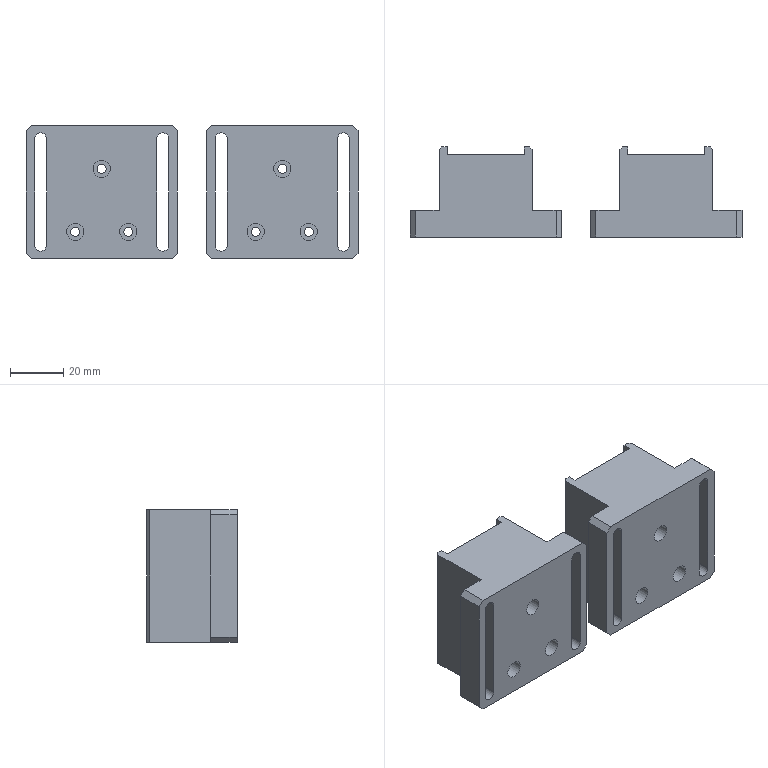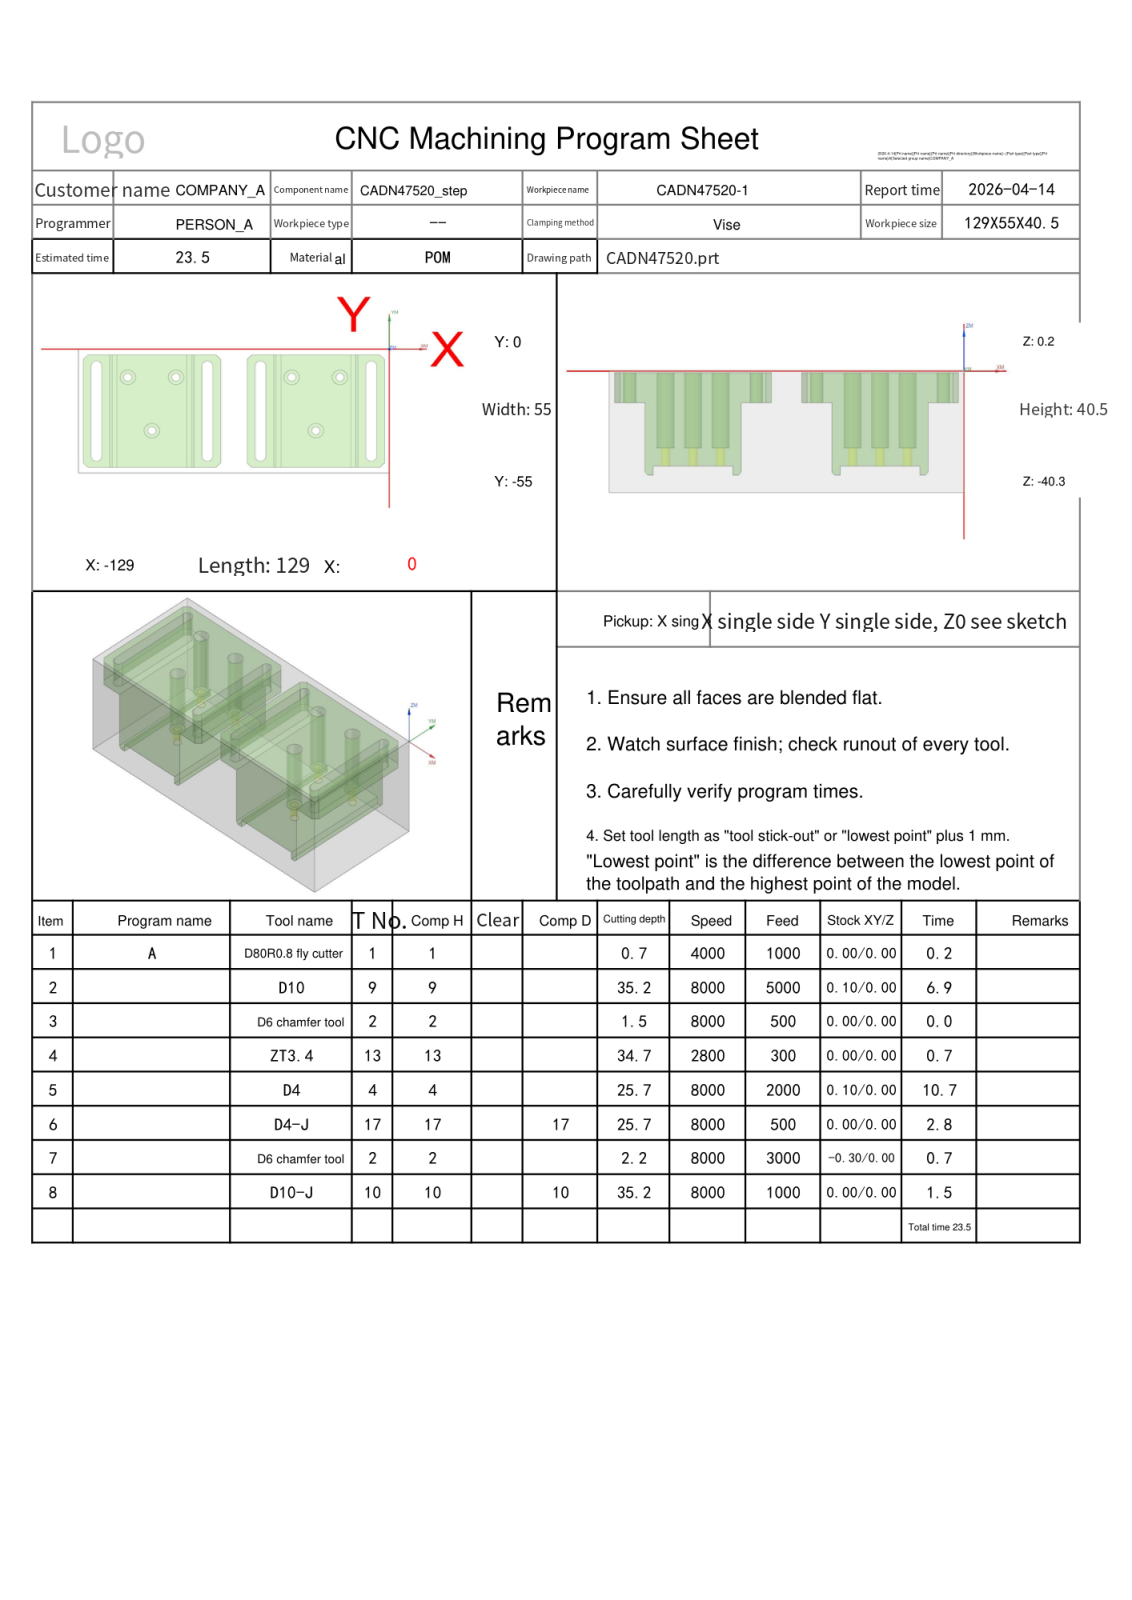NC program | NX | posted by the shop | part box 125 x 34 x 50 mm
Lines 2381 to 3331 of 5259:
N5 T04 M06
(D4  D=4. R=0. H=04 ce=0.10 di=0.10)
G00 G90 G54 X-7.65 Y-27.5 M03 S8000
G43 H04 Z19.5
M08
Z0.0
G01 Y-47.5 Z-.06 F2500.
G03 X-7.5 Y-47.65 Z-.061 I.15 J0.0
X-7.35 Y-47.5 Z-.062 I0.0 J.15
G01 Y-7.5 Z-.183
G03 X-7.5 Y-7.35 Z-.183 I-.15 J0.0
X-7.65 Y-7.5 Z-.184 I0.0 J-.15
G01 Y-47.5 Z-.305
G03 X-7.5 Y-47.65 Z-.306 I.15 J0.0
X-7.35 Y-47.5 Z-.306 I0.0 J.15
G01 Y-7.5 Z-.427
G03 X-7.5 Y-7.35 Z-.428 I-.15 J0.0
X-7.65 Y-7.5 Z-.428 I0.0 J-.15
G01 Y-47.5 Z-.549
G03 X-7.5 Y-47.65 Z-.55 I.15 J0.0
X-7.35 Y-47.5 Z-.551 I0.0 J.15
G01 Y-7.5 Z-.672
G03 X-7.5 Y-7.35 Z-.672 I-.15 J0.0
X-7.65 Y-7.5 Z-.673 I0.0 J-.15
G01 Y-47.5 Z-.794
G03 X-7.5 Y-47.65 Z-.794 I.15 J0.0
X-7.35 Y-47.5 Z-.795 I0.0 J.15
G01 Y-7.5 Z-.916
G03 X-7.5 Y-7.35 Z-.917 I-.15 J0.0
X-7.65 Y-7.5 Z-.917 I0.0 J-.15
G01 Y-47.5 Z-1.038
G03 X-7.5 Y-47.65 Z-1.039 I.15 J0.0
X-7.35 Y-47.5 Z-1.04 I0.0 J.15
G01 Y-7.5 Z-1.16
G03 X-7.5 Y-7.35 Z-1.161 I-.15 J0.0
X-7.65 Y-7.5 Z-1.162 I0.0 J-.15
G01 Y-47.5 Z-1.283
G03 X-7.5 Y-47.65 Z-1.283 I.15 J0.0
X-7.35 Y-47.5 Z-1.284 I0.0 J.15
G01 Y-7.5 Z-1.405
G03 X-7.5 Y-7.35 Z-1.406 I-.15 J0.0
X-7.65 Y-7.5 Z-1.406 I0.0 J-.15
G01 Y-47.5 Z-1.527
G03 X-7.5 Y-47.65 Z-1.528 I.15 J0.0
X-7.35 Y-47.5 Z-1.528 I0.0 J.15
G01 Y-7.5 Z-1.649
G03 X-7.5 Y-7.35 Z-1.65 I-.15 J0.0
X-7.65 Y-7.5 Z-1.651 I0.0 J-.15
G01 Y-47.5 Z-1.772
G03 X-7.5 Y-47.65 Z-1.772 I.15 J0.0
X-7.35 Y-47.5 Z-1.773 I0.0 J.15
G01 Y-7.5 Z-1.894
G03 X-7.5 Y-7.35 Z-1.894 I-.15 J0.0
X-7.65 Y-7.5 Z-1.895 I0.0 J-.15
G01 Y-47.5 Z-2.016
G03 X-7.5 Y-47.65 Z-2.017 I.15 J0.0
X-7.35 Y-47.5 Z-2.017 I0.0 J.15
G01 Y-7.5 Z-2.138
G03 X-7.5 Y-7.35 Z-2.139 I-.15 J0.0
X-7.65 Y-7.5 Z-2.14 I0.0 J-.15
G01 Y-47.5 Z-2.26
G03 X-7.5 Y-47.65 Z-2.261 I.15 J0.0
X-7.35 Y-47.5 Z-2.262 I0.0 J.15
G01 Y-7.5 Z-2.383
G03 X-7.5 Y-7.35 Z-2.383 I-.15 J0.0
X-7.65 Y-7.5 Z-2.384 I0.0 J-.15
G01 Y-47.5 Z-2.505
G03 X-7.5 Y-47.65 Z-2.506 I.15 J0.0
X-7.35 Y-47.5 Z-2.506 I0.0 J.15
G01 Y-7.5 Z-2.627
G03 X-7.5 Y-7.35 Z-2.628 I-.15 J0.0
X-7.65 Y-7.5 Z-2.628 I0.0 J-.15
G01 Y-47.5 Z-2.749
G03 X-7.5 Y-47.65 Z-2.75 I.15 J0.0
X-7.35 Y-47.5 Z-2.751 I0.0 J.15
G01 Y-7.5 Z-2.872
G03 X-7.5 Y-7.35 Z-2.872 I-.15 J0.0
X-7.65 Y-7.5 Z-2.873 I0.0 J-.15
G01 Y-47.5 Z-2.994
G03 X-7.5 Y-47.65 Z-2.994 I.15 J0.0
X-7.35 Y-47.5 Z-2.995 I0.0 J.15
G01 Y-7.5 Z-3.116
G03 X-7.5 Y-7.35 Z-3.117 I-.15 J0.0
X-7.65 Y-7.5 Z-3.117 I0.0 J-.15
G01 Y-47.5 Z-3.238
G03 X-7.5 Y-47.65 Z-3.239 I.15 J0.0
X-7.35 Y-47.5 Z-3.24 I0.0 J.15
G01 Y-7.5 Z-3.36
G03 X-7.5 Y-7.35 Z-3.361 I-.15 J0.0
X-7.65 Y-7.5 Z-3.362 I0.0 J-.15
G01 Y-47.5 Z-3.483
G03 X-7.5 Y-47.65 Z-3.483 I.15 J0.0
X-7.35 Y-47.5 Z-3.484 I0.0 J.15
G01 Y-7.5 Z-3.605
G03 X-7.5 Y-7.35 Z-3.606 I-.15 J0.0
X-7.65 Y-7.5 Z-3.606 I0.0 J-.15
G01 Y-47.5 Z-3.727
G03 X-7.5 Y-47.65 Z-3.728 I.15 J0.0
X-7.35 Y-47.5 Z-3.728 I0.0 J.15
G01 Y-7.5 Z-3.849
G03 X-7.5 Y-7.35 Z-3.85 I-.15 J0.0
X-7.65 Y-7.5 Z-3.851 I0.0 J-.15
G01 Y-47.5 Z-3.972
G03 X-7.5 Y-47.65 Z-3.972 I.15 J0.0
X-7.35 Y-47.5 Z-3.973 I0.0 J.15
G01 Y-7.5 Z-4.094
G03 X-7.5 Y-7.35 Z-4.094 I-.15 J0.0
X-7.65 Y-7.5 Z-4.095 I0.0 J-.15
G01 Y-47.5 Z-4.216
G03 X-7.5 Y-47.65 Z-4.217 I.15 J0.0
X-7.35 Y-47.5 Z-4.217 I0.0 J.15
G01 Y-7.5 Z-4.338
G03 X-7.5 Y-7.35 Z-4.339 I-.15 J0.0
X-7.65 Y-7.5 Z-4.34 I0.0 J-.15
G01 Y-47.5 Z-4.46
G03 X-7.5 Y-47.65 Z-4.461 I.15 J0.0
X-7.35 Y-47.5 Z-4.462 I0.0 J.15
G01 Y-7.5 Z-4.583
G03 X-7.5 Y-7.35 Z-4.583 I-.15 J0.0
X-7.65 Y-7.5 Z-4.584 I0.0 J-.15
G01 Y-47.5 Z-4.705
G03 X-7.5 Y-47.65 Z-4.706 I.15 J0.0
X-7.35 Y-47.5 Z-4.706 I0.0 J.15
G01 Y-7.5 Z-4.827
G03 X-7.5 Y-7.35 Z-4.828 I-.15 J0.0
X-7.65 Y-7.5 Z-4.828 I0.0 J-.15
G01 Y-47.5 Z-4.949
G03 X-7.5 Y-47.65 Z-4.95 I.15 J0.0
X-7.35 Y-47.5 Z-4.951 I0.0 J.15
G01 Y-7.5 Z-5.072
G03 X-7.5 Y-7.35 Z-5.072 I-.15 J0.0
X-7.65 Y-7.5 Z-5.073 I0.0 J-.15
G01 Y-47.5 Z-5.194
G03 X-7.5 Y-47.65 Z-5.194 I.15 J0.0
X-7.35 Y-47.5 Z-5.195 I0.0 J.15
G01 Y-7.5 Z-5.316
G03 X-7.5 Y-7.35 Z-5.317 I-.15 J0.0
X-7.65 Y-7.5 Z-5.317 I0.0 J-.15
G01 Y-47.5 Z-5.438
G03 X-7.5 Y-47.65 Z-5.439 I.15 J0.0
X-7.35 Y-47.5 Z-5.44 I0.0 J.15
G01 Y-7.5 Z-5.56
G03 X-7.5 Y-7.35 Z-5.561 I-.15 J0.0
X-7.65 Y-7.5 Z-5.562 I0.0 J-.15
G01 Y-47.5 Z-5.683
G03 X-7.5 Y-47.65 Z-5.683 I.15 J0.0
X-7.35 Y-47.5 Z-5.684 I0.0 J.15
G01 Y-7.5 Z-5.805
G03 X-7.5 Y-7.35 Z-5.806 I-.15 J0.0
X-7.65 Y-7.5 Z-5.806 I0.0 J-.15
G01 Y-47.5 Z-5.927
G03 X-7.5 Y-47.65 Z-5.928 I.15 J0.0
X-7.35 Y-47.5 Z-5.928 I0.0 J.15
G01 Y-7.5 Z-6.049
G03 X-7.5 Y-7.35 Z-6.05 I-.15 J0.0
X-7.65 Y-7.5 Z-6.051 I0.0 J-.15
G01 Y-47.5 Z-6.172
G03 X-7.5 Y-47.65 Z-6.172 I.15 J0.0
X-7.35 Y-47.5 Z-6.173 I0.0 J.15
G01 Y-7.5 Z-6.294
G03 X-7.5 Y-7.35 Z-6.294 I-.15 J0.0
X-7.65 Y-7.5 Z-6.295 I0.0 J-.15
G01 Y-47.5 Z-6.416
G03 X-7.5 Y-47.65 Z-6.417 I.15 J0.0
X-7.35 Y-47.5 Z-6.417 I0.0 J.15
G01 Y-7.5 Z-6.538
G03 X-7.5 Y-7.35 Z-6.539 I-.15 J0.0
X-7.65 Y-7.5 Z-6.54 I0.0 J-.15
G01 Y-47.5 Z-6.66
G03 X-7.5 Y-47.65 Z-6.661 I.15 J0.0
X-7.35 Y-47.5 Z-6.662 I0.0 J.15
G01 Y-7.5 Z-6.783
G03 X-7.5 Y-7.35 Z-6.783 I-.15 J0.0
X-7.65 Y-7.5 Z-6.784 I0.0 J-.15
G01 Y-47.5 Z-6.905
G03 X-7.5 Y-47.65 Z-6.906 I.15 J0.0
X-7.35 Y-47.5 Z-6.906 I0.0 J.15
G01 Y-7.5 Z-7.027
G03 X-7.5 Y-7.35 Z-7.028 I-.15 J0.0
X-7.65 Y-7.5 Z-7.028 I0.0 J-.15
G01 Y-47.5 Z-7.149
G03 X-7.5 Y-47.65 Z-7.15 I.15 J0.0
X-7.35 Y-47.5 Z-7.151 I0.0 J.15
G01 Y-7.5 Z-7.272
G03 X-7.5 Y-7.35 Z-7.272 I-.15 J0.0
X-7.65 Y-7.5 Z-7.273 I0.0 J-.15
G01 Y-47.5 Z-7.394
G03 X-7.5 Y-47.65 Z-7.394 I.15 J0.0
X-7.35 Y-47.5 Z-7.395 I0.0 J.15
G01 Y-7.5 Z-7.516
G03 X-7.5 Y-7.35 Z-7.517 I-.15 J0.0
X-7.65 Y-7.5 Z-7.517 I0.0 J-.15
G01 Y-47.5 Z-7.638
G03 X-7.5 Y-47.65 Z-7.639 I.15 J0.0
X-7.35 Y-47.5 Z-7.64 I0.0 J.15
G01 Y-7.5 Z-7.76
G03 X-7.5 Y-7.35 Z-7.761 I-.15 J0.0
X-7.65 Y-7.5 Z-7.762 I0.0 J-.15
G01 Y-47.5 Z-7.883
G03 X-7.5 Y-47.65 Z-7.883 I.15 J0.0
X-7.35 Y-47.5 Z-7.884 I0.0 J.15
G01 Y-7.5 Z-8.005
G03 X-7.5 Y-7.35 Z-8.006 I-.15 J0.0
X-7.65 Y-7.5 Z-8.006 I0.0 J-.15
G01 Y-47.5 Z-8.127
G03 X-7.5 Y-47.65 Z-8.128 I.15 J0.0
X-7.35 Y-47.5 Z-8.128 I0.0 J.15
G01 Y-7.5 Z-8.249
G03 X-7.5 Y-7.35 Z-8.25 I-.15 J0.0
X-7.65 Y-7.5 Z-8.251 I0.0 J-.15
G01 Y-47.5 Z-8.372
G03 X-7.5 Y-47.65 Z-8.372 I.15 J0.0
X-7.35 Y-47.5 Z-8.373 I0.0 J.15
G01 Y-7.5 Z-8.494
G03 X-7.5 Y-7.35 Z-8.494 I-.15 J0.0
X-7.65 Y-7.5 Z-8.495 I0.0 J-.15
G01 Y-47.5 Z-8.616
G03 X-7.5 Y-47.65 Z-8.617 I.15 J0.0
X-7.35 Y-47.5 Z-8.617 I0.0 J.15
G01 Y-7.5 Z-8.738
G03 X-7.5 Y-7.35 Z-8.739 I-.15 J0.0
X-7.65 Y-7.5 Z-8.74 I0.0 J-.15
G01 Y-47.5 Z-8.86
G03 X-7.5 Y-47.65 Z-8.861 I.15 J0.0
X-7.35 Y-47.5 Z-8.862 I0.0 J.15
G01 Y-7.5 Z-8.983
G03 X-7.5 Y-7.35 Z-8.983 I-.15 J0.0
X-7.65 Y-7.5 Z-8.984 I0.0 J-.15
G01 Y-47.5 Z-9.105
G03 X-7.5 Y-47.65 Z-9.106 I.15 J0.0
X-7.35 Y-47.5 Z-9.106 I0.0 J.15
G01 Y-7.5 Z-9.227
G03 X-7.5 Y-7.35 Z-9.228 I-.15 J0.0
X-7.65 Y-7.5 Z-9.228 I0.0 J-.15
G01 Y-47.5 Z-9.349
G03 X-7.5 Y-47.65 Z-9.35 I.15 J0.0
X-7.35 Y-47.5 Z-9.351 I0.0 J.15
G01 Y-7.5 Z-9.472
G03 X-7.5 Y-7.35 Z-9.472 I-.15 J0.0
X-7.65 Y-7.5 Z-9.473 I0.0 J-.15
G01 Y-47.5 Z-9.594
G03 X-7.5 Y-47.65 Z-9.594 I.15 J0.0
X-7.35 Y-47.5 Z-9.595 I0.0 J.15
G01 Y-7.5 Z-9.716
G03 X-7.5 Y-7.35 Z-9.717 I-.15 J0.0
X-7.65 Y-7.5 Z-9.717 I0.0 J-.15
G01 Y-47.5 Z-9.838
G03 X-7.5 Y-47.65 Z-9.839 I.15 J0.0
X-7.35 Y-47.5 Z-9.84 I0.0 J.15
G01 Y-7.5 Z-9.96
G03 X-7.5 Y-7.35 Z-9.961 I-.15 J0.0
X-7.65 Y-7.5 Z-9.962 I0.0 J-.15
G01 Y-47.5 Z-10.083
G03 X-7.5 Y-47.65 Z-10.083 I.15 J0.0
X-7.35 Y-47.5 Z-10.084 I0.0 J.15
G01 Y-7.5 Z-10.205
G03 X-7.5 Y-7.35 Z-10.206 I-.15 J0.0
X-7.65 Y-7.5 Z-10.206 I0.0 J-.15
G01 Y-47.5 Z-10.327
G03 X-7.5 Y-47.65 Z-10.328 I.15 J0.0
X-7.35 Y-47.5 Z-10.328 I0.0 J.15
G01 Y-7.5 Z-10.449
G03 X-7.5 Y-7.35 Z-10.45 I-.15 J0.0
X-7.65 Y-7.5 Z-10.451 I0.0 J-.15
G01 Y-47.5 Z-10.572
G03 X-7.5 Y-47.65 Z-10.572 I.15 J0.0
X-7.35 Y-47.5 Z-10.573 I0.0 J.15
G01 Y-7.5 Z-10.694
G03 X-7.5 Y-7.35 Z-10.694 I-.15 J0.0
X-7.65 Y-7.5 Z-10.695 I0.0 J-.15
G01 Y-47.5 Z-10.816
G03 X-7.5 Y-47.65 Z-10.817 I.15 J0.0
X-7.35 Y-47.5 Z-10.817 I0.0 J.15
G01 Y-7.5 Z-10.938
G03 X-7.5 Y-7.35 Z-10.939 I-.15 J0.0
X-7.65 Y-7.5 Z-10.94 I0.0 J-.15
G01 Y-27.5 Z-11.
Y-47.5
G03 X-7.5 Y-47.65 I.15 J0.0
X-7.35 Y-47.5 I0.0 J.15
G01 Y-7.5
G03 X-7.5 Y-7.35 I-.15 J0.0
X-7.65 Y-7.5 I0.0 J-.15
G01 Y-27.5
Y-28.
Z-10.
G00 Z19.5
X-53.65 Y-27.5
Z0.0
G01 Y-47.5 Z-.06
G03 X-53.5 Y-47.65 Z-.061 I.15 J0.0
X-53.35 Y-47.5 Z-.062 I0.0 J.15
G01 Y-7.5 Z-.183
Y-7.445
X-53.378 Y-7.397
X-53.425 Y-7.37
X-53.459 Y-7.345
X-53.5 Y-7.35
G03 X-53.65 Y-7.5 Z-.184 I0.0 J-.15
G01 Y-47.5 Z-.305
G03 X-53.5 Y-47.65 Z-.306 I.15 J0.0
X-53.35 Y-47.5 Z-.306 I0.0 J.15
G01 Y-7.5 Z-.427
Y-7.445
X-53.378 Y-7.397
X-53.425 Y-7.37 Z-.428
X-53.459 Y-7.345
X-53.5 Y-7.35
G03 X-53.65 Y-7.5 Z-.428 I0.0 J-.15
G01 Y-47.5 Z-.549
G03 X-53.5 Y-47.65 Z-.55 I.15 J0.0
X-53.35 Y-47.5 Z-.551 I0.0 J.15
G01 Y-7.5 Z-.672
Y-7.445
X-53.378 Y-7.397
X-53.425 Y-7.37
X-53.459 Y-7.345
X-53.5 Y-7.35
G03 X-53.65 Y-7.5 Z-.673 I0.0 J-.15
G01 Y-47.5 Z-.794
G03 X-53.5 Y-47.65 Z-.794 I.15 J0.0
X-53.35 Y-47.5 Z-.795 I0.0 J.15
G01 Y-7.5 Z-.916
Y-7.445
X-53.378 Y-7.397
X-53.425 Y-7.37
X-53.459 Y-7.345 Z-.917
X-53.5 Y-7.35
G03 X-53.65 Y-7.5 Z-.917 I0.0 J-.15
G01 Y-47.5 Z-1.038
G03 X-53.5 Y-47.65 Z-1.039 I.15 J0.0
X-53.35 Y-47.5 Z-1.04 I0.0 J.15
G01 Y-7.5 Z-1.16
Y-7.445 Z-1.161
X-53.378 Y-7.397
X-53.425 Y-7.37
X-53.459 Y-7.345
X-53.5 Y-7.35
G03 X-53.65 Y-7.5 Z-1.162 I0.0 J-.15
G01 Y-47.5 Z-1.283
G03 X-53.5 Y-47.65 Z-1.283 I.15 J0.0
X-53.35 Y-47.5 Z-1.284 I0.0 J.15
G01 Y-7.5 Z-1.405
Y-7.445
X-53.378 Y-7.397
X-53.425 Y-7.37
X-53.459 Y-7.345
X-53.5 Y-7.35 Z-1.406
G03 X-53.65 Y-7.5 Z-1.406 I0.0 J-.15
G01 Y-47.5 Z-1.527
G03 X-53.5 Y-47.65 Z-1.528 I.15 J0.0
X-53.35 Y-47.5 Z-1.528 I0.0 J.15
G01 Y-7.5 Z-1.649
Y-7.445
X-53.378 Y-7.397 Z-1.65
X-53.425 Y-7.37
X-53.459 Y-7.345
X-53.5 Y-7.35
G03 X-53.65 Y-7.5 Z-1.651 I0.0 J-.15
G01 Y-47.5 Z-1.772
G03 X-53.5 Y-47.65 Z-1.772 I.15 J0.0
X-53.35 Y-47.5 Z-1.773 I0.0 J.15
G01 Y-7.5 Z-1.894
Y-7.445
X-53.378 Y-7.397
X-53.425 Y-7.37
X-53.459 Y-7.345
X-53.5 Y-7.35
G03 X-53.65 Y-7.5 Z-1.895 I0.0 J-.15
G01 Y-47.5 Z-2.016
G03 X-53.5 Y-47.65 Z-2.017 I.15 J0.0
X-53.35 Y-47.5 Z-2.017 I0.0 J.15
G01 Y-7.5 Z-2.138
Y-7.445
X-53.378 Y-7.397
X-53.425 Y-7.37 Z-2.139
X-53.459 Y-7.345
X-53.5 Y-7.35
G03 X-53.65 Y-7.5 Z-2.14 I0.0 J-.15
G01 Y-47.5 Z-2.26
G03 X-53.5 Y-47.65 Z-2.261 I.15 J0.0
X-53.35 Y-47.5 Z-2.262 I0.0 J.15
G01 Y-7.5 Z-2.383
Y-7.445
X-53.378 Y-7.397
X-53.425 Y-7.37
X-53.459 Y-7.345
X-53.5 Y-7.35
G03 X-53.65 Y-7.5 Z-2.384 I0.0 J-.15
G01 Y-47.5 Z-2.505
G03 X-53.5 Y-47.65 Z-2.506 I.15 J0.0
X-53.35 Y-47.5 Z-2.506 I0.0 J.15
G01 Y-7.5 Z-2.627
Y-7.445
X-53.378 Y-7.397
X-53.425 Y-7.37 Z-2.628
X-53.459 Y-7.345
X-53.5 Y-7.35
G03 X-53.65 Y-7.5 Z-2.628 I0.0 J-.15
G01 Y-47.5 Z-2.749
G03 X-53.5 Y-47.65 Z-2.75 I.15 J0.0
X-53.35 Y-47.5 Z-2.751 I0.0 J.15
G01 Y-7.5 Z-2.872
Y-7.445
X-53.378 Y-7.397
X-53.425 Y-7.37
X-53.459 Y-7.345
X-53.5 Y-7.35
G03 X-53.65 Y-7.5 Z-2.873 I0.0 J-.15
G01 Y-47.5 Z-2.994
G03 X-53.5 Y-47.65 Z-2.994 I.15 J0.0
X-53.35 Y-47.5 Z-2.995 I0.0 J.15
G01 Y-7.5 Z-3.116
Y-7.445
X-53.378 Y-7.397
X-53.425 Y-7.37
X-53.459 Y-7.345 Z-3.117
X-53.5 Y-7.35
G03 X-53.65 Y-7.5 Z-3.117 I0.0 J-.15
G01 Y-47.5 Z-3.238
G03 X-53.5 Y-47.65 Z-3.239 I.15 J0.0
X-53.35 Y-47.5 Z-3.24 I0.0 J.15
G01 Y-7.5 Z-3.36
Y-7.445 Z-3.361
X-53.378 Y-7.397
X-53.425 Y-7.37
X-53.459 Y-7.345
X-53.5 Y-7.35
G03 X-53.65 Y-7.5 Z-3.362 I0.0 J-.15
G01 Y-47.5 Z-3.483
G03 X-53.5 Y-47.65 Z-3.483 I.15 J0.0
X-53.35 Y-47.5 Z-3.484 I0.0 J.15
G01 Y-7.5 Z-3.605
Y-7.445
X-53.378 Y-7.397
X-53.425 Y-7.37
X-53.459 Y-7.345
X-53.5 Y-7.35 Z-3.606
G03 X-53.65 Y-7.5 Z-3.606 I0.0 J-.15
G01 Y-47.5 Z-3.727
G03 X-53.5 Y-47.65 Z-3.728 I.15 J0.0
X-53.35 Y-47.5 Z-3.728 I0.0 J.15
G01 Y-7.5 Z-3.849
Y-7.445
X-53.378 Y-7.397 Z-3.85
X-53.425 Y-7.37
X-53.459 Y-7.345
X-53.5 Y-7.35
G03 X-53.65 Y-7.5 Z-3.851 I0.0 J-.15
G01 Y-47.5 Z-3.972
G03 X-53.5 Y-47.65 Z-3.972 I.15 J0.0
X-53.35 Y-47.5 Z-3.973 I0.0 J.15
G01 Y-7.5 Z-4.094
Y-7.445
X-53.378 Y-7.397
X-53.425 Y-7.37
X-53.459 Y-7.345
X-53.5 Y-7.35
G03 X-53.65 Y-7.5 Z-4.095 I0.0 J-.15
G01 Y-47.5 Z-4.216
G03 X-53.5 Y-47.65 Z-4.217 I.15 J0.0
X-53.35 Y-47.5 Z-4.217 I0.0 J.15
G01 Y-7.5 Z-4.338
Y-7.445
X-53.378 Y-7.397
X-53.425 Y-7.37 Z-4.339
X-53.459 Y-7.345
X-53.5 Y-7.35
G03 X-53.65 Y-7.5 Z-4.34 I0.0 J-.15
G01 Y-47.5 Z-4.46
G03 X-53.5 Y-47.65 Z-4.461 I.15 J0.0
X-53.35 Y-47.5 Z-4.462 I0.0 J.15
G01 Y-7.5 Z-4.583
Y-7.445
X-53.378 Y-7.397
X-53.425 Y-7.37
X-53.459 Y-7.345
X-53.5 Y-7.35
G03 X-53.65 Y-7.5 Z-4.584 I0.0 J-.15
G01 Y-47.5 Z-4.705
G03 X-53.5 Y-47.65 Z-4.706 I.15 J0.0
X-53.35 Y-47.5 Z-4.706 I0.0 J.15
G01 Y-7.5 Z-4.827
Y-7.445
X-53.378 Y-7.397
X-53.425 Y-7.37 Z-4.828
X-53.459 Y-7.345
X-53.5 Y-7.35
G03 X-53.65 Y-7.5 Z-4.828 I0.0 J-.15
G01 Y-47.5 Z-4.949
G03 X-53.5 Y-47.65 Z-4.95 I.15 J0.0
X-53.35 Y-47.5 Z-4.951 I0.0 J.15
G01 Y-7.5 Z-5.072
Y-7.445
X-53.378 Y-7.397
X-53.425 Y-7.37
X-53.459 Y-7.345
X-53.5 Y-7.35
G03 X-53.65 Y-7.5 Z-5.073 I0.0 J-.15
G01 Y-47.5 Z-5.194
G03 X-53.5 Y-47.65 Z-5.194 I.15 J0.0
X-53.35 Y-47.5 Z-5.195 I0.0 J.15
G01 Y-7.5 Z-5.316
Y-7.445
X-53.378 Y-7.397
X-53.425 Y-7.37
X-53.459 Y-7.345 Z-5.317
X-53.5 Y-7.35
G03 X-53.65 Y-7.5 Z-5.317 I0.0 J-.15
G01 Y-47.5 Z-5.438
G03 X-53.5 Y-47.65 Z-5.439 I.15 J0.0
X-53.35 Y-47.5 Z-5.44 I0.0 J.15
G01 Y-7.5 Z-5.56
Y-7.445 Z-5.561
X-53.378 Y-7.397
X-53.425 Y-7.37
X-53.459 Y-7.345
X-53.5 Y-7.35
G03 X-53.65 Y-7.5 Z-5.562 I0.0 J-.15
G01 Y-47.5 Z-5.683
G03 X-53.5 Y-47.65 Z-5.683 I.15 J0.0
X-53.35 Y-47.5 Z-5.684 I0.0 J.15
G01 Y-7.5 Z-5.805
Y-7.445
X-53.378 Y-7.397
X-53.425 Y-7.37
X-53.459 Y-7.345
X-53.5 Y-7.35 Z-5.806
G03 X-53.65 Y-7.5 Z-5.806 I0.0 J-.15
G01 Y-47.5 Z-5.927
G03 X-53.5 Y-47.65 Z-5.928 I.15 J0.0
X-53.35 Y-47.5 Z-5.928 I0.0 J.15
G01 Y-7.5 Z-6.049
Y-7.445
X-53.378 Y-7.397 Z-6.05
X-53.425 Y-7.37
X-53.459 Y-7.345
X-53.5 Y-7.35
G03 X-53.65 Y-7.5 Z-6.051 I0.0 J-.15
G01 Y-47.5 Z-6.172
G03 X-53.5 Y-47.65 Z-6.172 I.15 J0.0
X-53.35 Y-47.5 Z-6.173 I0.0 J.15
G01 Y-7.5 Z-6.294
Y-7.445
X-53.378 Y-7.397
X-53.425 Y-7.37
X-53.459 Y-7.345
X-53.5 Y-7.35
G03 X-53.65 Y-7.5 Z-6.295 I0.0 J-.15
G01 Y-47.5 Z-6.416
G03 X-53.5 Y-47.65 Z-6.417 I.15 J0.0
X-53.35 Y-47.5 Z-6.417 I0.0 J.15
G01 Y-7.5 Z-6.538
Y-7.445
X-53.378 Y-7.397
X-53.425 Y-7.37 Z-6.539
X-53.459 Y-7.345
X-53.5 Y-7.35
G03 X-53.65 Y-7.5 Z-6.54 I0.0 J-.15
G01 Y-47.5 Z-6.66
G03 X-53.5 Y-47.65 Z-6.661 I.15 J0.0
X-53.35 Y-47.5 Z-6.662 I0.0 J.15
G01 Y-7.5 Z-6.783
Y-7.445
X-53.378 Y-7.397
X-53.425 Y-7.37
X-53.459 Y-7.345
X-53.5 Y-7.35
G03 X-53.65 Y-7.5 Z-6.784 I0.0 J-.15
G01 Y-47.5 Z-6.905
G03 X-53.5 Y-47.65 Z-6.906 I.15 J0.0
X-53.35 Y-47.5 Z-6.906 I0.0 J.15
G01 Y-7.5 Z-7.027
Y-7.445
X-53.378 Y-7.397
X-53.425 Y-7.37 Z-7.028
X-53.459 Y-7.345
X-53.5 Y-7.35
G03 X-53.65 Y-7.5 Z-7.028 I0.0 J-.15
G01 Y-47.5 Z-7.149
G03 X-53.5 Y-47.65 Z-7.15 I.15 J0.0
X-53.35 Y-47.5 Z-7.151 I0.0 J.15
G01 Y-7.5 Z-7.272
Y-7.445
X-53.378 Y-7.397
X-53.425 Y-7.37
X-53.459 Y-7.345
X-53.5 Y-7.35
G03 X-53.65 Y-7.5 Z-7.273 I0.0 J-.15
G01 Y-47.5 Z-7.394
G03 X-53.5 Y-47.65 Z-7.394 I.15 J0.0
X-53.35 Y-47.5 Z-7.395 I0.0 J.15
G01 Y-7.5 Z-7.516
Y-7.445
X-53.378 Y-7.397
X-53.425 Y-7.37
X-53.459 Y-7.345 Z-7.517
X-53.5 Y-7.35
G03 X-53.65 Y-7.5 Z-7.517 I0.0 J-.15
G01 Y-47.5 Z-7.638
G03 X-53.5 Y-47.65 Z-7.639 I.15 J0.0
X-53.35 Y-47.5 Z-7.64 I0.0 J.15
G01 Y-7.5 Z-7.76
Y-7.445 Z-7.761
X-53.378 Y-7.397
X-53.425 Y-7.37
X-53.459 Y-7.345
X-53.5 Y-7.35
G03 X-53.65 Y-7.5 Z-7.762 I0.0 J-.15
G01 Y-47.5 Z-7.883
G03 X-53.5 Y-47.65 Z-7.883 I.15 J0.0
X-53.35 Y-47.5 Z-7.884 I0.0 J.15
G01 Y-7.5 Z-8.005
Y-7.445
X-53.378 Y-7.397
X-53.425 Y-7.37
X-53.459 Y-7.345
X-53.5 Y-7.35 Z-8.006
G03 X-53.65 Y-7.5 Z-8.006 I0.0 J-.15
G01 Y-47.5 Z-8.127
G03 X-53.5 Y-47.65 Z-8.128 I.15 J0.0
X-53.35 Y-47.5 Z-8.128 I0.0 J.15
G01 Y-7.5 Z-8.249
Y-7.445
X-53.378 Y-7.397 Z-8.25
X-53.425 Y-7.37
X-53.459 Y-7.345
X-53.5 Y-7.35
G03 X-53.65 Y-7.5 Z-8.251 I0.0 J-.15
G01 Y-47.5 Z-8.372
G03 X-53.5 Y-47.65 Z-8.372 I.15 J0.0
X-53.35 Y-47.5 Z-8.373 I0.0 J.15
G01 Y-7.5 Z-8.494
Y-7.445
X-53.378 Y-7.397
X-53.425 Y-7.37
X-53.459 Y-7.345
X-53.5 Y-7.35
G03 X-53.65 Y-7.5 Z-8.495 I0.0 J-.15
G01 Y-47.5 Z-8.616
G03 X-53.5 Y-47.65 Z-8.617 I.15 J0.0
X-53.35 Y-47.5 Z-8.617 I0.0 J.15
G01 Y-7.5 Z-8.738
Y-7.445
X-53.378 Y-7.397
X-53.425 Y-7.37 Z-8.739
X-53.459 Y-7.345
X-53.5 Y-7.35
G03 X-53.65 Y-7.5 Z-8.74 I0.0 J-.15
G01 Y-47.5 Z-8.86
G03 X-53.5 Y-47.65 Z-8.861 I.15 J0.0
X-53.35 Y-47.5 Z-8.862 I0.0 J.15
G01 Y-7.5 Z-8.983
Y-7.445
X-53.378 Y-7.397
X-53.425 Y-7.37
X-53.459 Y-7.345
X-53.5 Y-7.35
G03 X-53.65 Y-7.5 Z-8.984 I0.0 J-.15
G01 Y-47.5 Z-9.105
G03 X-53.5 Y-47.65 Z-9.106 I.15 J0.0
X-53.35 Y-47.5 Z-9.106 I0.0 J.15
G01 Y-7.5 Z-9.227
Y-7.445
X-53.378 Y-7.397
X-53.425 Y-7.37 Z-9.228
X-53.459 Y-7.345
X-53.5 Y-7.35
G03 X-53.65 Y-7.5 Z-9.228 I0.0 J-.15
G01 Y-47.5 Z-9.349
G03 X-53.5 Y-47.65 Z-9.35 I.15 J0.0
X-53.35 Y-47.5 Z-9.351 I0.0 J.15
G01 Y-7.5 Z-9.472
Y-7.445
X-53.378 Y-7.397
X-53.425 Y-7.37
X-53.459 Y-7.345
X-53.5 Y-7.35
G03 X-53.65 Y-7.5 Z-9.473 I0.0 J-.15
G01 Y-47.5 Z-9.594
G03 X-53.5 Y-47.65 Z-9.594 I.15 J0.0
X-53.35 Y-47.5 Z-9.595 I0.0 J.15
G01 Y-7.5 Z-9.716
Y-7.445
X-53.378 Y-7.397
X-53.425 Y-7.37
X-53.459 Y-7.345 Z-9.717
X-53.5 Y-7.35
G03 X-53.65 Y-7.5 Z-9.717 I0.0 J-.15
G01 Y-47.5 Z-9.838
G03 X-53.5 Y-47.65 Z-9.839 I.15 J0.0
X-53.35 Y-47.5 Z-9.84 I0.0 J.15
G01 Y-7.5 Z-9.96
Y-7.445 Z-9.961
X-53.378 Y-7.397
X-53.425 Y-7.37
X-53.459 Y-7.345
X-53.5 Y-7.35
G03 X-53.65 Y-7.5 Z-9.962 I0.0 J-.15
G01 Y-47.5 Z-10.083
G03 X-53.5 Y-47.65 Z-10.083 I.15 J0.0
X-53.35 Y-47.5 Z-10.084 I0.0 J.15
G01 Y-7.5 Z-10.205
Y-7.445
X-53.378 Y-7.397
X-53.425 Y-7.37
X-53.459 Y-7.345
X-53.5 Y-7.35 Z-10.206
G03 X-53.65 Y-7.5 Z-10.206 I0.0 J-.15
G01 Y-47.5 Z-10.327
G03 X-53.5 Y-47.65 Z-10.328 I.15 J0.0
X-53.35 Y-47.5 Z-10.328 I0.0 J.15
G01 Y-7.5 Z-10.449
Y-7.445
X-53.378 Y-7.397 Z-10.45
X-53.425 Y-7.37
X-53.459 Y-7.345
X-53.5 Y-7.35
G03 X-53.65 Y-7.5 Z-10.451 I0.0 J-.15
G01 Y-47.5 Z-10.572
G03 X-53.5 Y-47.65 Z-10.572 I.15 J0.0
X-53.35 Y-47.5 Z-10.573 I0.0 J.15
G01 Y-7.5 Z-10.694
Y-7.445
X-53.378 Y-7.397
X-53.425 Y-7.37
X-53.459 Y-7.345
X-53.5 Y-7.35
G03 X-53.65 Y-7.5 Z-10.695 I0.0 J-.15
G01 Y-47.5 Z-10.816
G03 X-53.5 Y-47.65 Z-10.817 I.15 J0.0
X-53.35 Y-47.5 Z-10.817 I0.0 J.15
G01 Y-7.5 Z-10.938
Y-7.445
X-53.378 Y-7.397
X-53.425 Y-7.37 Z-10.939
X-53.459 Y-7.345
X-53.5 Y-7.35
G03 X-53.65 Y-7.5 Z-10.94 I0.0 J-.15
G01 Y-27.5 Z-11.
Y-47.5
G03 X-53.5 Y-47.65 I.15 J0.0
X-53.35 Y-47.5 I0.0 J.15
G01 Y-7.5
G03 X-53.5 Y-7.35 I-.15 J0.0
X-53.65 Y-7.5 I0.0 J-.15
G01 Y-27.5
Y-28.
Z-10.
G00 Z19.5
X-75.65 Y-27.5
Z0.0
G01 Y-47.5 Z-.06
G03 X-75.5 Y-47.65 Z-.061 I.15 J0.0
X-75.35 Y-47.5 Z-.062 I0.0 J.15
G01 Y-7.5 Z-.183
G03 X-75.5 Y-7.35 Z-.183 I-.15 J0.0
X-75.65 Y-7.5 Z-.184 I0.0 J-.15
G01 Y-47.5 Z-.305
G03 X-75.5 Y-47.65 Z-.306 I.15 J0.0
X-75.35 Y-47.5 Z-.306 I0.0 J.15
G01 Y-7.5 Z-.427
G03 X-75.5 Y-7.35 Z-.428 I-.15 J0.0
X-75.65 Y-7.5 Z-.428 I0.0 J-.15
G01 Y-47.5 Z-.549
G03 X-75.5 Y-47.65 Z-.55 I.15 J0.0
X-75.35 Y-47.5 Z-.551 I0.0 J.15
G01 Y-7.5 Z-.672
G03 X-75.5 Y-7.35 Z-.672 I-.15 J0.0
X-75.65 Y-7.5 Z-.673 I0.0 J-.15
G01 Y-47.5 Z-.794
G03 X-75.5 Y-47.65 Z-.794 I.15 J0.0
X-75.35 Y-47.5 Z-.795 I0.0 J.15
G01 Y-7.5 Z-.916
G03 X-75.5 Y-7.35 Z-.917 I-.15 J0.0
X-75.65 Y-7.5 Z-.917 I0.0 J-.15
G01 Y-47.5 Z-1.038
G03 X-75.5 Y-47.65 Z-1.039 I.15 J0.0
X-75.35 Y-47.5 Z-1.04 I0.0 J.15
G01 Y-7.5 Z-1.16
G03 X-75.5 Y-7.35 Z-1.161 I-.15 J0.0
X-75.65 Y-7.5 Z-1.162 I0.0 J-.15
G01 Y-47.5 Z-1.283
G03 X-75.5 Y-47.65 Z-1.283 I.15 J0.0
X-75.35 Y-47.5 Z-1.284 I0.0 J.15
G01 Y-7.5 Z-1.405
G03 X-75.5 Y-7.35 Z-1.406 I-.15 J0.0
X-75.65 Y-7.5 Z-1.406 I0.0 J-.15
G01 Y-47.5 Z-1.527
G03 X-75.5 Y-47.65 Z-1.528 I.15 J0.0
X-75.35 Y-47.5 Z-1.528 I0.0 J.15
G01 Y-7.5 Z-1.649
G03 X-75.5 Y-7.35 Z-1.65 I-.15 J0.0
X-75.65 Y-7.5 Z-1.651 I0.0 J-.15
G01 Y-47.5 Z-1.772
G03 X-75.5 Y-47.65 Z-1.772 I.15 J0.0
X-75.35 Y-47.5 Z-1.773 I0.0 J.15
G01 Y-7.5 Z-1.894
G03 X-75.5 Y-7.35 Z-1.894 I-.15 J0.0
X-75.65 Y-7.5 Z-1.895 I0.0 J-.15
G01 Y-47.5 Z-2.016
G03 X-75.5 Y-47.65 Z-2.017 I.15 J0.0
X-75.35 Y-47.5 Z-2.017 I0.0 J.15
G01 Y-7.5 Z-2.138
G03 X-75.5 Y-7.35 Z-2.139 I-.15 J0.0
X-75.65 Y-7.5 Z-2.14 I0.0 J-.15
G01 Y-47.5 Z-2.26
G03 X-75.5 Y-47.65 Z-2.261 I.15 J0.0
X-75.35 Y-47.5 Z-2.262 I0.0 J.15
G01 Y-7.5 Z-2.383
G03 X-75.5 Y-7.35 Z-2.383 I-.15 J0.0
X-75.65 Y-7.5 Z-2.384 I0.0 J-.15
G01 Y-47.5 Z-2.505
G03 X-75.5 Y-47.65 Z-2.506 I.15 J0.0
X-75.35 Y-47.5 Z-2.506 I0.0 J.15
G01 Y-7.5 Z-2.627
G03 X-75.5 Y-7.35 Z-2.628 I-.15 J0.0
X-75.65 Y-7.5 Z-2.628 I0.0 J-.15
G01 Y-47.5 Z-2.749
G03 X-75.5 Y-47.65 Z-2.75 I.15 J0.0
X-75.35 Y-47.5 Z-2.751 I0.0 J.15
G01 Y-7.5 Z-2.872
G03 X-75.5 Y-7.35 Z-2.872 I-.15 J0.0
X-75.65 Y-7.5 Z-2.873 I0.0 J-.15
G01 Y-47.5 Z-2.994
G03 X-75.5 Y-47.65 Z-2.994 I.15 J0.0
X-75.35 Y-47.5 Z-2.995 I0.0 J.15
G01 Y-7.5 Z-3.116
G03 X-75.5 Y-7.35 Z-3.117 I-.15 J0.0
X-75.65 Y-7.5 Z-3.117 I0.0 J-.15
G01 Y-47.5 Z-3.238
G03 X-75.5 Y-47.65 Z-3.239 I.15 J0.0
X-75.35 Y-47.5 Z-3.24 I0.0 J.15
G01 Y-7.5 Z-3.36
G03 X-75.5 Y-7.35 Z-3.361 I-.15 J0.0
X-75.65 Y-7.5 Z-3.362 I0.0 J-.15
G01 Y-47.5 Z-3.483
G03 X-75.5 Y-47.65 Z-3.483 I.15 J0.0
X-75.35 Y-47.5 Z-3.484 I0.0 J.15
G01 Y-7.5 Z-3.605
G03 X-75.5 Y-7.35 Z-3.606 I-.15 J0.0
X-75.65 Y-7.5 Z-3.606 I0.0 J-.15
G01 Y-47.5 Z-3.727
G03 X-75.5 Y-47.65 Z-3.728 I.15 J0.0
X-75.35 Y-47.5 Z-3.728 I0.0 J.15
G01 Y-7.5 Z-3.849
G03 X-75.5 Y-7.35 Z-3.85 I-.15 J0.0
X-75.65 Y-7.5 Z-3.851 I0.0 J-.15
G01 Y-47.5 Z-3.972
G03 X-75.5 Y-47.65 Z-3.972 I.15 J0.0
X-75.35 Y-47.5 Z-3.973 I0.0 J.15
G01 Y-7.5 Z-4.094
G03 X-75.5 Y-7.35 Z-4.094 I-.15 J0.0
X-75.65 Y-7.5 Z-4.095 I0.0 J-.15
G01 Y-47.5 Z-4.216
G03 X-75.5 Y-47.65 Z-4.217 I.15 J0.0
X-75.35 Y-47.5 Z-4.217 I0.0 J.15
G01 Y-7.5 Z-4.338
G03 X-75.5 Y-7.35 Z-4.339 I-.15 J0.0
X-75.65 Y-7.5 Z-4.34 I0.0 J-.15
G01 Y-47.5 Z-4.46
G03 X-75.5 Y-47.65 Z-4.461 I.15 J0.0
X-75.35 Y-47.5 Z-4.462 I0.0 J.15
G01 Y-7.5 Z-4.583
G03 X-75.5 Y-7.35 Z-4.583 I-.15 J0.0
X-75.65 Y-7.5 Z-4.584 I0.0 J-.15
G01 Y-47.5 Z-4.705
G03 X-75.5 Y-47.65 Z-4.706 I.15 J0.0
X-75.35 Y-47.5 Z-4.706 I0.0 J.15
G01 Y-7.5 Z-4.827
G03 X-75.5 Y-7.35 Z-4.828 I-.15 J0.0
X-75.65 Y-7.5 Z-4.828 I0.0 J-.15
G01 Y-47.5 Z-4.949
G03 X-75.5 Y-47.65 Z-4.95 I.15 J0.0
X-75.35 Y-47.5 Z-4.951 I0.0 J.15
G01 Y-7.5 Z-5.072
G03 X-75.5 Y-7.35 Z-5.072 I-.15 J0.0
X-75.65 Y-7.5 Z-5.073 I0.0 J-.15
G01 Y-47.5 Z-5.194
G03 X-75.5 Y-47.65 Z-5.194 I.15 J0.0
X-75.35 Y-47.5 Z-5.195 I0.0 J.15
G01 Y-7.5 Z-5.316
G03 X-75.5 Y-7.35 Z-5.317 I-.15 J0.0
X-75.65 Y-7.5 Z-5.317 I0.0 J-.15
G01 Y-47.5 Z-5.438
G03 X-75.5 Y-47.65 Z-5.439 I.15 J0.0
X-75.35 Y-47.5 Z-5.44 I0.0 J.15
G01 Y-7.5 Z-5.56
G03 X-75.5 Y-7.35 Z-5.561 I-.15 J0.0
X-75.65 Y-7.5 Z-5.562 I0.0 J-.15
G01 Y-47.5 Z-5.683
G03 X-75.5 Y-47.65 Z-5.683 I.15 J0.0
X-75.35 Y-47.5 Z-5.684 I0.0 J.15
G01 Y-7.5 Z-5.805
G03 X-75.5 Y-7.35 Z-5.806 I-.15 J0.0
X-75.65 Y-7.5 Z-5.806 I0.0 J-.15
G01 Y-47.5 Z-5.927
G03 X-75.5 Y-47.65 Z-5.928 I.15 J0.0
X-75.35 Y-47.5 Z-5.928 I0.0 J.15
G01 Y-7.5 Z-6.049
G03 X-75.5 Y-7.35 Z-6.05 I-.15 J0.0
X-75.65 Y-7.5 Z-6.051 I0.0 J-.15
G01 Y-47.5 Z-6.172
G03 X-75.5 Y-47.65 Z-6.172 I.15 J0.0
X-75.35 Y-47.5 Z-6.173 I0.0 J.15
G01 Y-7.5 Z-6.294
G03 X-75.5 Y-7.35 Z-6.294 I-.15 J0.0
X-75.65 Y-7.5 Z-6.295 I0.0 J-.15
G01 Y-47.5 Z-6.416
G03 X-75.5 Y-47.65 Z-6.417 I.15 J0.0
X-75.35 Y-47.5 Z-6.417 I0.0 J.15
G01 Y-7.5 Z-6.538
G03 X-75.5 Y-7.35 Z-6.539 I-.15 J0.0
X-75.65 Y-7.5 Z-6.54 I0.0 J-.15
G01 Y-47.5 Z-6.66
G03 X-75.5 Y-47.65 Z-6.661 I.15 J0.0
X-75.35 Y-47.5 Z-6.662 I0.0 J.15
G01 Y-7.5 Z-6.783
G03 X-75.5 Y-7.35 Z-6.783 I-.15 J0.0
X-75.65 Y-7.5 Z-6.784 I0.0 J-.15
G01 Y-47.5 Z-6.905
G03 X-75.5 Y-47.65 Z-6.906 I.15 J0.0
X-75.35 Y-47.5 Z-6.906 I0.0 J.15
G01 Y-7.5 Z-7.027
G03 X-75.5 Y-7.35 Z-7.028 I-.15 J0.0
X-75.65 Y-7.5 Z-7.028 I0.0 J-.15
G01 Y-47.5 Z-7.149
G03 X-75.5 Y-47.65 Z-7.15 I.15 J0.0
X-75.35 Y-47.5 Z-7.151 I0.0 J.15
G01 Y-7.5 Z-7.272
G03 X-75.5 Y-7.35 Z-7.272 I-.15 J0.0
X-75.65 Y-7.5 Z-7.273 I0.0 J-.15
G01 Y-47.5 Z-7.394
G03 X-75.5 Y-47.65 Z-7.394 I.15 J0.0
X-75.35 Y-47.5 Z-7.395 I0.0 J.15
G01 Y-7.5 Z-7.516
G03 X-75.5 Y-7.35 Z-7.517 I-.15 J0.0
X-75.65 Y-7.5 Z-7.517 I0.0 J-.15
G01 Y-47.5 Z-7.638
G03 X-75.5 Y-47.65 Z-7.639 I.15 J0.0
X-75.35 Y-47.5 Z-7.64 I0.0 J.15
G01 Y-7.5 Z-7.76
G03 X-75.5 Y-7.35 Z-7.761 I-.15 J0.0
X-75.65 Y-7.5 Z-7.762 I0.0 J-.15
G01 Y-47.5 Z-7.883
G03 X-75.5 Y-47.65 Z-7.883 I.15 J0.0
X-75.35 Y-47.5 Z-7.884 I0.0 J.15
G01 Y-7.5 Z-8.005
G03 X-75.5 Y-7.35 Z-8.006 I-.15 J0.0
X-75.65 Y-7.5 Z-8.006 I0.0 J-.15
G01 Y-47.5 Z-8.127